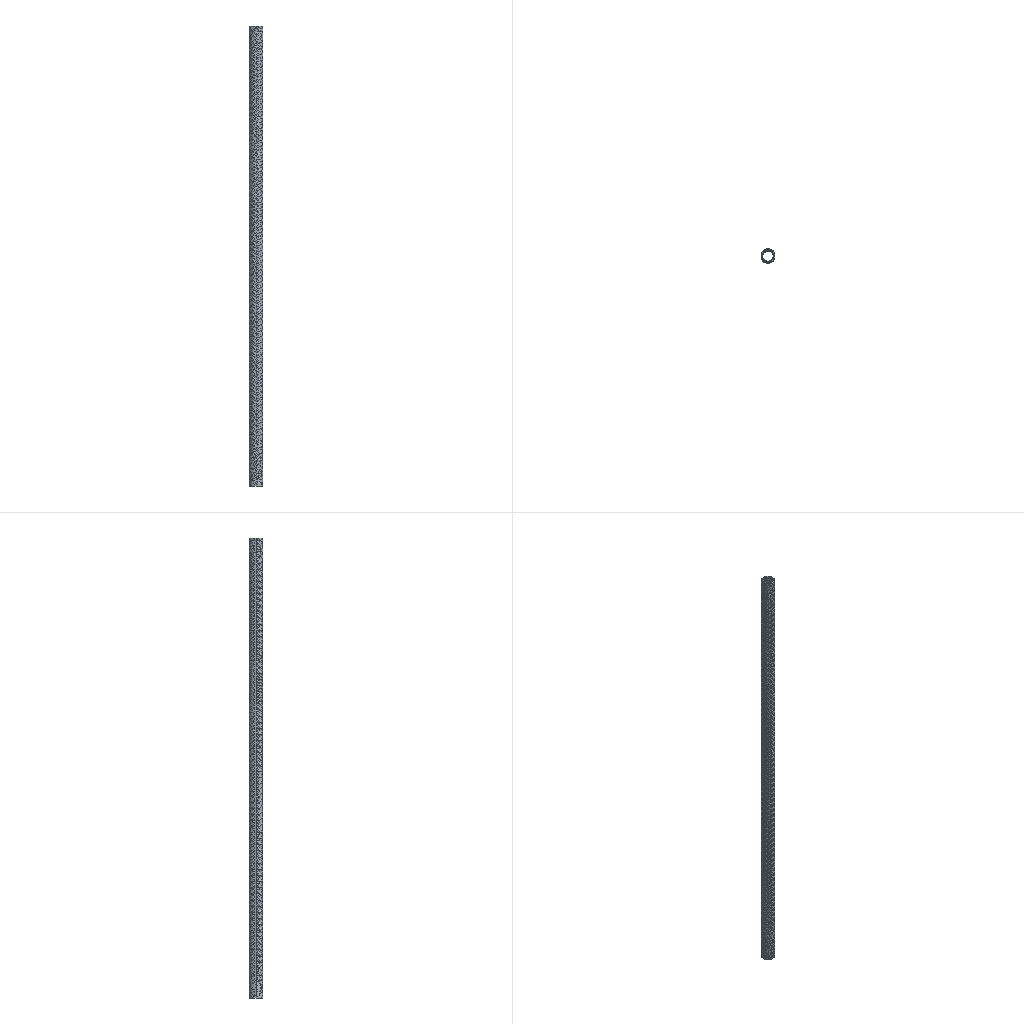Simulation study | ansys workbench
Ansys APDL input file, long lists of numbers shortened:
/batch
/config,noeldb,1     ! force off writing results to database
*get,_wallstrt,active,,time,wall
! ANSYS input file written by Workbench version 2022 R1
! File used for geometry attach: F:\ansys（分析文件汇总)\ansys刀片有限元分析\装配体\长杆.STEP
/title,2222--____ (C5)
! ****** Begin Custom Load Command Snippet ******
/COM, ACT Extensions:
/COM,     LSDYNA, 2021.1
/COM,
! ****** End   Custom Load Command Snippet ******
*DIM,_wb_ProjectScratch_dir,string,248
_wb_ProjectScratch_dir(1) = 'F:\ansys（分析文件汇总)\ansys刀片有限元分析\_ProjectScratch\Scr367D\'
*DIM,_wb_SolverFiles_dir,string,248
_wb_SolverFiles_dir(1) = 'F:\ansys（分析文件汇总)\ansys刀片有限元分析\2222_files\dp0\SYS-1\MECH\'
*DIM,_wb_userfiles_dir,string,248
_wb_userfiles_dir(1) = 'F:\ansys（分析文件汇总)\ansys刀片有限元分析\2222_files\user_files\'
/com,--- Data in consistent NMM units. See Solving Units in the help system for more information.
/units,MPA
/nopr
/wb,file,start              !  signify a WB generated input file
/prep7
! Turn off shape checking because checks already performed inside WB mesher.
! See help system for more information.
SHPP,OFF,,NOWARN
/nolist
etcon,set             ! allow ANSYS to choose best KEYOP's for 180x elements, resets any applicable keyopt to MAPDL defaults
/com,*********** Nodes for the whole assembly ***********
nblock,3,,32644
(1i9,3e20.9e3)
        1     2.250000000E+01     2.755455298E-15    -2.500000000E+02
! (29676 more lines like these left out)
-1
/com,*********** Nodes for all Remote Points ***********
nblock,3
(1i9,3e20.9e3)
    29678    -5.505508782E-16     1.776356839E-15    -1.000000000E+03
-1
/wb,elem,start            !  set before creation of elements
/com,*********** Elements for Body 1 "__-FreeParts|__-__1" ***********
et,1,187
eblock,19,solid,,14973
(19i9)
        1        1        1        1        0        0        0        0       10        0        1      197      543     4110      198     6610     9348     6616     6608
! (29945 more lines like these left out)
-1
/wb,elem,end               !  done creating elements
/com,*********** Send User Defined Coordinate System(s) ***********
csys,0
toffst,273.15,  ! Temperature offset from absolute zero
/com,*********** Set Reference Temperature ***********
tref,22.
/wb,mat,start              !  starting to send materials
/com,*********** Send Materials ***********
Temperature = 'TEMP' ! Temperature
MP,DENS,1,7.85e-09,	! tonne mm^-3
MP,ALPX,1,1.2e-05,	! C^-1
MP,C,1,434000000,	! mm^2 s^-2 C^-1
MP,KXX,1,60.5,	! tonne mm s^-3 C^-1
MP,RSVX,1,0.00017,	! ohm mm
MP,EX,1,200000,	! tonne s^-2 mm^-1
MP,NUXY,1,0.3,
MP,MURX,1,10000,
/wb,mat,end                !  done sending materials
!************************* Model Summary ********************
!__-FreeParts|__-__1,	结构钢,	matid,	1
!************************* End Model Summary ********************
! get the diagonal of the bounding box. Needed later for other things
*get,_xmin,node,,mnloc,x
*get,_ymin,node,,mnloc,y
*get,_zmin,node,,mnloc,z
*get,_xmax,node,,mxloc,x
*get,_ymax,node,,mxloc,y
*get,_zmax,node,,mxloc,z
_ASMDIAG=(_xmax-_xmin)*(_xmax-_xmin)+(_ymax-_ymin)*(_ymax-_ymin)+(_zmax-_zmin)*(_zmax-_zmin)
_ASMDIAG=SQRT(_ASMDIAG)
/wb,contact,start          !  starting to send contact
/wb,contact,end            !  done creating contacts
/golist
/wb,load,start             !  starting to send loads
/com,*********** Fixed Supports ***********
CMBLOCK,_FIXEDSU,NODE,      192
(8i10)
         1         2         3         4         5         6         7         8
! (23 more lines like these left out)
cmsel,s,_FIXEDSU
d,all,all
nsel,all
/com,*********** Create Remote Point "内部远程点" ***********
! -------- Remote Point Used by "力矩" --------
*set,tid,3
*set,cid,2
et,cid,174
et,tid,170
keyo,tid,2,1               ! Don't fix the pilot node
keyo,tid,4,111111
keyo,cid,12,5              ! Bonded Contact
keyo,cid,4,1               ! Deformable RBE3 style load
keyo,cid,2,2               ! MPC style contact
eblock,10,,,4544
(15i9)
    24767        2        2        2        0      179      180     3073     3073     6461     6474     3073     6466
! (4543 more lines like these left out)
-1
*set,_npilot,29678
_npilot32=_npilot
type,tid
mat ,cid
real,cid
tshape,pilo
en,29311,_npilot
tshape
/com,*********** Construct Moment Using Remote Attachment ***********
/gst,on,on
fini
*get,_numnode,node,0,count
*get,_numelem,elem,0,count
*get, _MAXELEMNUM, elem, 0, NUM, MAX
*get, _MAXNODENUM, node, 0, NUM, MAX
*get, _MAXELEMTYPE, etyp, 0, NUM, MAX
*get, _MAXREALCONST, real, 0, NUM, MAX
/go
/wb,load,end               !  done creating loads
/com,--- Number of total nodes = %_numnode%
/com,--- Number of contact elements = 4544
/com,--- Number of spring elements = 0
/com,--- Number of bearing elements = 0
/com,--- Number of solid elements = 14973
/com,--- Number of condensed parts = 0
/com,--- Number of total elements = %_numelem%
*get,_wallbsol,active,,time,wall
/com,****************************************************************************
/com,*************************    SOLUTION       ********************************
/com,****************************************************************************
/solu
antype,0                   ! static analysis
_thickRatio=  0     ! Ratio of thick parts in the model
eqsl,sparse,,,,,1
cntr,print,1               ! print out contact info and also make no initial contact an error
dmpoption,emat,no             ! Don't combine emat file for DANSYS
dmpoption,esav,no             ! Don't combine esav file for DANSYS
nldiag,cont,iter           ! print out contact info each equilibrium iteration
rescontrol,,none                 ! Do not keep any restart files
/com,****************************************************
/com,******************* SOLVE FOR LS 1 OF 1 ****************
nsel,s,node,,29678
f,all,mx,0.
f,all,my,0.
f,all,mz,800000.
nsel,all
/nopr
/gopr
nsub,1,1,1
time,1.
outres,erase
outres,all,none
outres,nsol,all,
outres,rsol,all
outres,eangl,all
outres,etmp,all
outres,veng,all
outres,strs,all,
outres,epel,all,
outres,eppl,all,
outres,cont,all,
! *********** WB SOLVE COMMAND ***********
! check interactive state
*get,ANSINTER_,active,,int
*if,ANSINTER_,ne,0,then
/eof
*endif
solve
/com *************** Write FE CONNECTORS *********
CEWRITE,file,ce,,INTE
/com,****************************************************
/com,*************** FINISHED SOLVE FOR LS 1 *************
*get,_wallasol,active,,time,wall
/nopr
*get,_numnode,node,0,count
*get,_numelem,elem,0,count
*get, _MAXELEMNUM, elem, 0, NUM, MAX
*get, _MAXNODENUM, node, 0, NUM, MAX,,,INTERNAL
*get, _MAXELEMTYPE, etyp, 0, NUM, MAX
*get, _MAXREALCONST, real, 0, NUM, MAX
/gopr
/post1
xmlo,ENCODING,ISO-8859-1
xmlo,parm
/xml,parm,xml
fini
/gopr
*get,_walldone,active,,time,wall
_preptime=(_wallbsol-_wallstrt)*3600
_solvtime=(_wallasol-_wallbsol)*3600
_posttime=(_walldone-_wallasol)*3600
_totaltim=(_walldone-_wallstrt)*3600
*get,_dlbratio,active,0,solu,dlbr
*get,_combtime,active,0,solu,comb
*get,_ssmode,active,0,solu,ssmm
*get,_ndofs,active,0,solu,ndof
*get,_sol_end_time,active,0,set,time
*if,_sol_end_time,eq,1.,then
/fclean				!clean distributed files
*endif
/com,--- Total number of nodes = %_numnode%
/com,--- Total number of elements = %_numelem%
/com,--- Element load balance ratio = %_dlbratio%
/com,--- Time to combine distributed files = %_combtime%
/com,--- Sparse memory mode = %_ssmode%
/com,--- Number of DOF = %_ndofs%
/wb,file,end               ! done with WB generated input